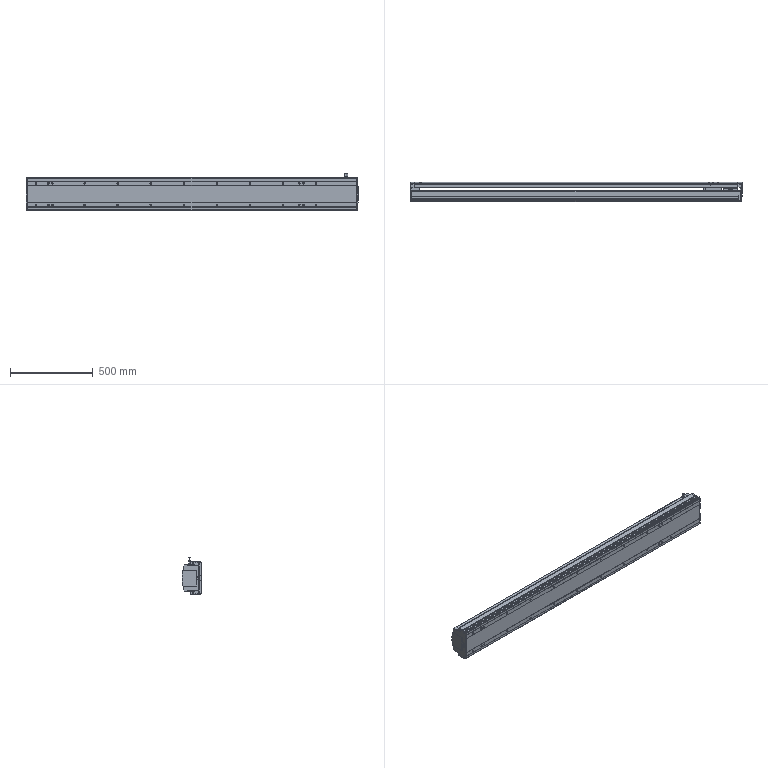Part | STEP file | ISB-WXMX-WA-750-25-1500-T4-N-A1-AQ-EB-^-Part-1 | 1 solid | 537 faces | box 2010 x 118.5 x 223.4 mm | volume 26600724 mm3 | plane 322 | cylinder 215 | commonest cylinder face diameters 9 x52 16 x36 8 x32 7 x16 7.6 x16 6 x12